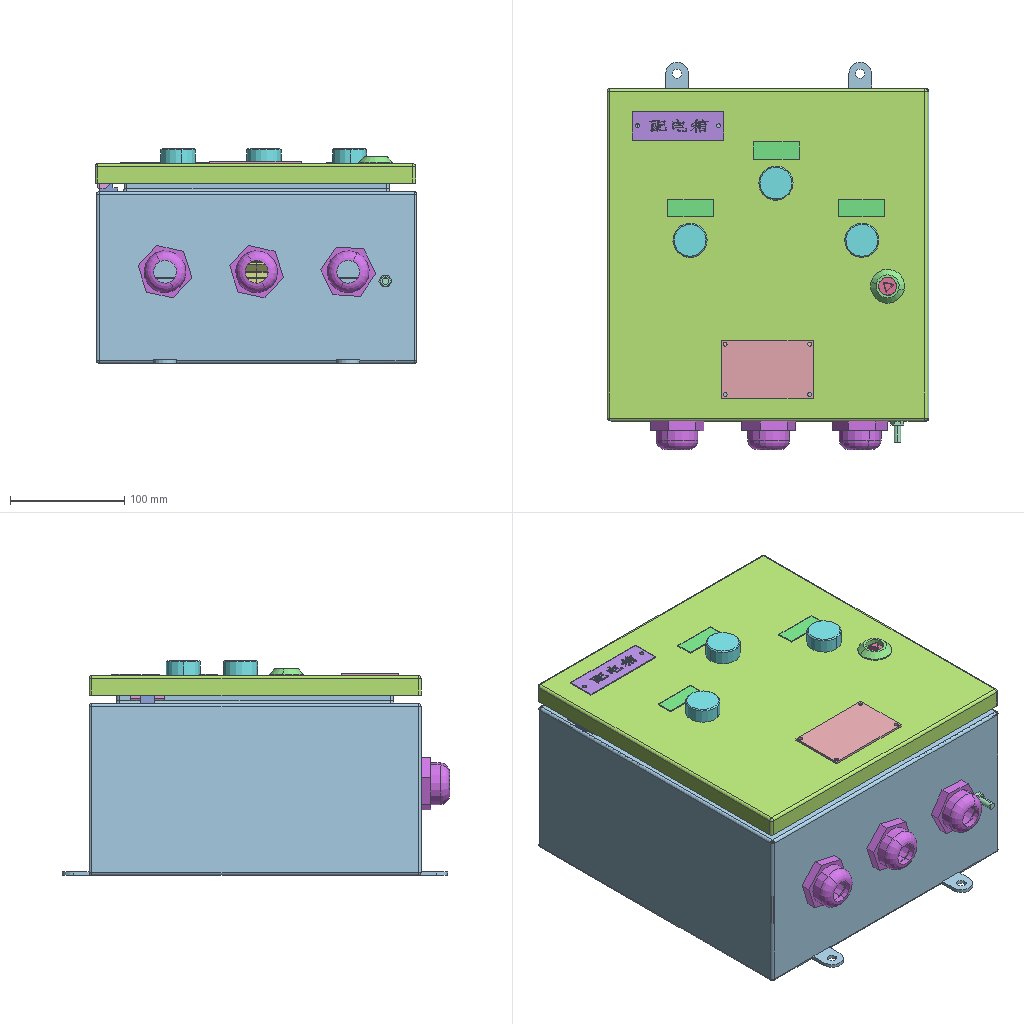Assembly | SolidWorks | 19 different items | 32 placed | box 281 x 338 x 188 mm
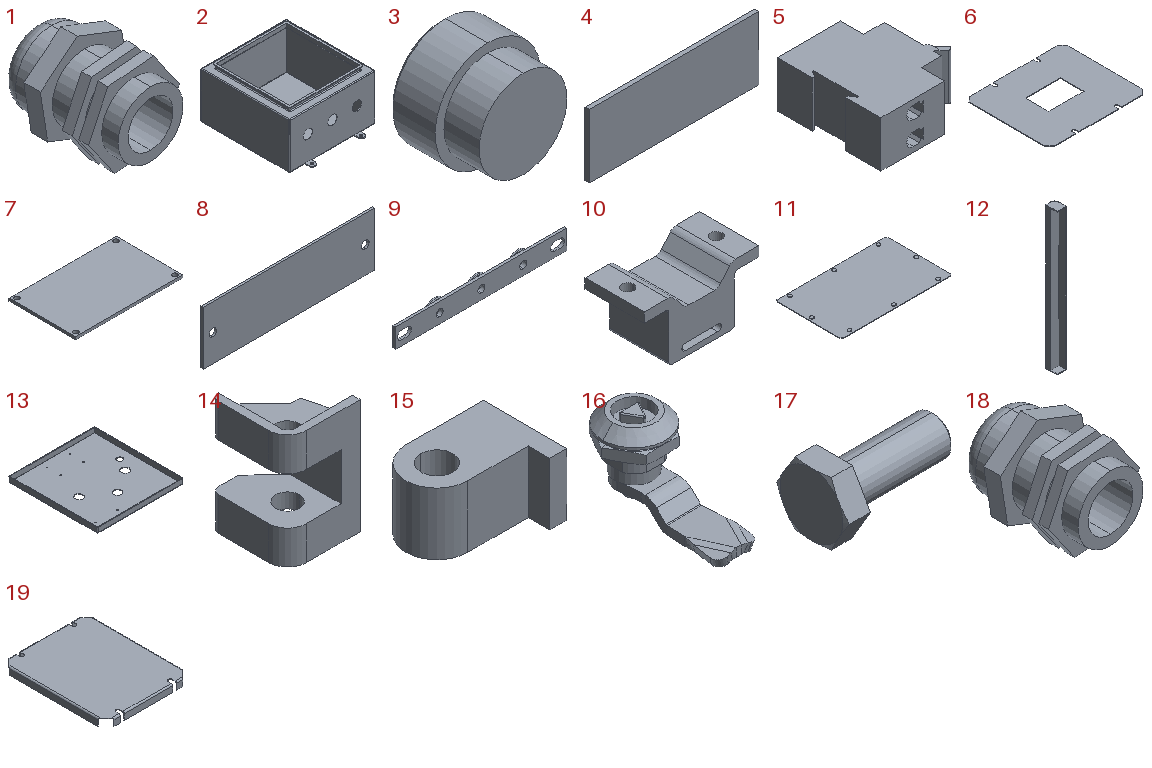Parts list (item | quantity | size | volume | features):
1 | x1 | 27.604 x 35 x 28.514 mm | 7936 mm3 | features ICE 5, Extrusion 1, Fillet 1, Shell 1
2 | x1 | 280 x 337 x 164.57 mm | 438435 mm3 | features ICE 4, Fillet 2, Extrusion 1, Shell 1
3 | x3 | 30 x 23 x 30 mm | 14052 mm3 | features Chamfer 1, Extrusion 1, ICE 1
4 | x3 | 40 x 1 x 15 mm | 600 mm3 | features Extrusion 1
5 | x2 | 74.887 x 81 x 36 mm | 158863 mm3 | features ICE 7, ConnectionPoint 4, Chamfer 1, CombineBodies 1, Extrusion 1, Fillet 1, LPattern 1, MirrorPattern 1, PLine 1
6 | x1 | 209.129 x 181.357 x 1.2 mm | 40439 mm3 | features ICE 6, MoveFace 2, BaseBody 1, Chamfer 1
7 | x1 | 80 x 50 x 2 mm | 7923 mm3 | features ICE 19, MoveFace 6, Fillet 2, BaseBody 1
8 | x1 | 80 x 1 x 25 mm | 1928 mm3 | features Extrusion 1, ICE 1
9 | x1 | 123 x 4 x 15 mm | 4060 mm3 | features ICE 2, Extrusion 1
10 | x1 | 70 x 36 x 40.002 mm | 44732 mm3 | features Fillet 3, ICE 3, Extrusion 1, HoleWzd 1
11 | x1 | 298 x 178 x 2.7 mm | 64049 mm3 | features BaseBody 9
12 | x1 | 19 x 24 x 298 mm | 61282 mm3 | features BaseBody 1
13 | x1 | 280 x 290 x 17.2 mm | 191799 mm3 | features ICE 17, MoveFace 7, Fillet 2, BaseBody 1
14 | x1 | 19 x 20 x 30 mm | 3284 mm3 | features BaseBody 1
15 | x1 | 21 x 16.2 x 12 mm | 2422 mm3 | features BaseBody 1
16 | x1 | 31.177 x 64.298 x 36.976 mm | 13076 mm3 | features BaseBody 5
17 | x7 | 18.975 x 11.258 x 9.75 mm | 741.836 mm3 | features BaseBody 1, MoveFace 1, Scale 1
18 | x3 | 46.006 x 58.333 x 47.523 mm | 36742 mm3 | features ICE 5, Extrusion 1, Fillet 1, Scale 1, Shell 1
19 | x1 | 148 x 182 x 12.6 mm | 38112 mm3 | features MoveFace 2, BaseBody 1
Mates (type | each side: item.copy, entity, surface, feature):
Coincident | 5.1 face plane Pattern(Linear)2 | 5.2 face plane Split Line4
Coincident | 5.1 face plane Boss-Extrude1 | 5.2 face plane Boss-Extrude1 | 2 times
Coincident | 2.1 face plane Boss-Extrude1 | 17.1 face plane Imported1
Coincident | 2.1 face plane Shell1 | 9.1 face plane Boss-Extrude1
Coincident | 2.1 face plane Shell1 | 17.2 face plane Imported1
Concentric | 19.1 edge | 17.2 face cylinder Imported1
Coincident | 2.1 face plane Shell1 | 17.3 face plane Imported1
Concentric | 19.1 edge | 17.3 face cylinder Imported1
Coincident | 2.1 face plane Shell1 | 17.4 face plane Imported1
Concentric | 19.1 edge | 17.4 face cylinder Imported1
Coincident | 2.1 face plane Shell1 | 17.5 face plane Imported1
Concentric | 19.1 edge | 17.5 face cylinder Imported1
Concentric | 2.1 edge | 18.1 face cylinder Boss-Extrude1
Coincident | 2.1 face plane Boss-Extrude1 | 18.1 face plane Boss-Extrude2
Coincident | 2.1 face plane Shell1 | 17.6 face plane Imported1
Coincident | 19.1 face plane Imported1 | 2.1 face plane Shell1
DistanceDim | 2.1 face plane Shell1 | 19.1 face plane Imported1 | 2 times
Coincident | 19.1 face plane Imported1 | 5.2 face plane Boss-Extrude1
DistanceDim | 2.1 face plane Shell1 | 5.2 face plane Boss-Extrude1
DistanceDim | 5.1 face plane Split Line4 | 2.1 face plane Shell1
Concentric | 2.1 face cylinder Cut-Extrude1 | 18.2 face cylinder Boss-Extrude1
Coincident | 2.1 face plane Boss-Extrude1 | 18.2 face plane Boss-Extrude2
Concentric | 2.1 face cylinder Cut-Extrude1 | 18.3 face cylinder Boss-Extrude1
Concentric | 13.1 face cylinder Imported1 | 16.1 face cylinder Input 4
Coincident | 13.1 face plane Imported1 | 16.1 face plane Input 4
Concentric | 15.1 face cylinder Input 1 | 14.1 face cylinder Input 1
Coincident | 15.1 face plane Input 1 | 14.1 face plane Input 1
Coincident | 13.1 face plane Imported1 | 14.1 face plane Input 1 | 2 times
Coincident | 15.1 face plane Input 1 | 2.1 face plane Boss-Extrude1
Coincident | 15.1 edge | 2.1 edge
Coincident | 13.1 face plane Imported1 | 2.1 face plane Boss-Extrude1
Parallel | 13.1 face plane Imported1 | 2.1 face plane Boss-Extrude1
Coincident | 2.1 face plane Boss-Extrude1 | 18.3 face plane Boss-Extrude2
Coincident | 13.1 face plane Imported1 | 17.7 face plane Imported1
Concentric | 13.1 edge | 3.1 face cylinder Boss-Extrude1
Coincident | 13.1 face plane Imported1 | 3.1 face plane Boss-Extrude1
Concentric | 13.1 face cylinder Cut-Extrude8 | 3.2 face cylinder Boss-Extrude1
Coincident | 13.1 face plane Imported1 | 3.2 face plane Boss-Extrude1
Concentric | 13.1 face cylinder Cut-Extrude8 | 3.3 face cylinder Boss-Extrude1
Coincident | 13.1 face plane Imported1 | 3.3 face plane Boss-Extrude1
Concentric | 17.2 face cylinder Imported1 | 6.1 edge
Concentric | 17.3 face cylinder Imported1 | 6.1 edge
Coincident | 13.1 face plane Imported1 | 8.1 face plane Boss-Extrude1
Concentric | 13.1 face cylinder Cut-Extrude9 | 8.1 face cylinder Boss-Extrude1 | 2 times
Coincident | 13.1 face plane Imported1 | 4.1 face plane Boss-Extrude1
Coincident | 13.1 face plane Imported1 | 4.2 face plane Boss-Extrude1
Coincident | 13.1 face plane Imported1 | 4.3 face plane Boss-Extrude1
Parallel | 13.1 face plane Imported1 | 4.1 face plane Boss-Extrude1
Parallel | 4.1 face plane Boss-Extrude1 | 4.2 face plane Boss-Extrude1
Parallel | 4.2 face plane Boss-Extrude1 | 4.3 face plane Boss-Extrude1
Coincident | 4.2 face plane Boss-Extrude1 | 4.3 face plane Boss-Extrude1
Coincident | 13.1 face plane Imported1 | 7.1 face plane Boss-Extrude12
Concentric | 13.1 face cylinder Cut-Extrude7 | 7.1 face cylinder Boss-Extrude12 | 2 times